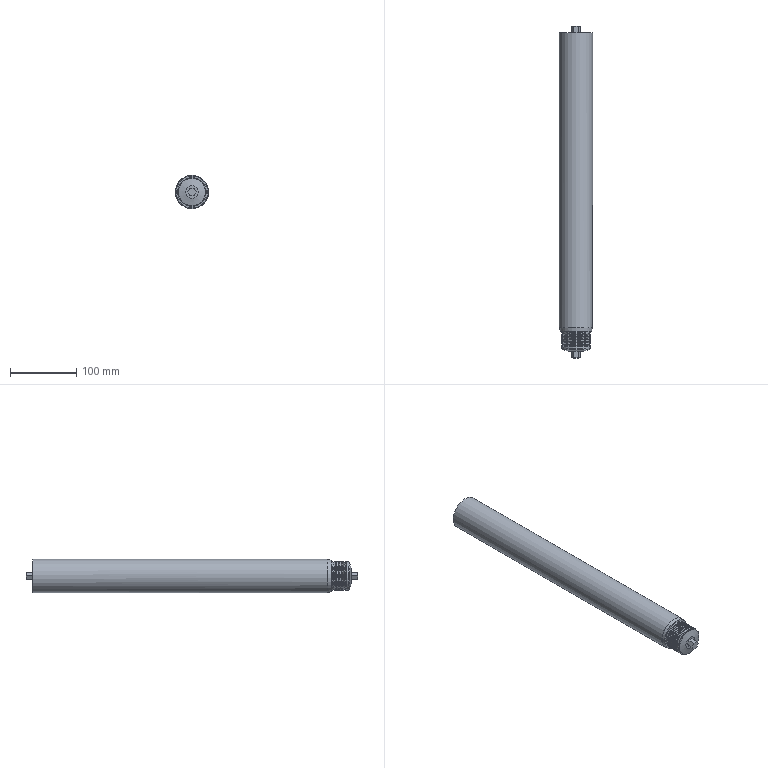Part | STEP file | Drive roller PolyV 420 mm | 1 solid | 71 faces | box 49.999 x 500 x 49.999 mm | volume 924230 mm3 | cone 28 | torus 20 | plane 19 | cylinder 4 | commonest cylinder face diameters 40.962 x1 43.299 x1 43.3 x1 49.999 x1